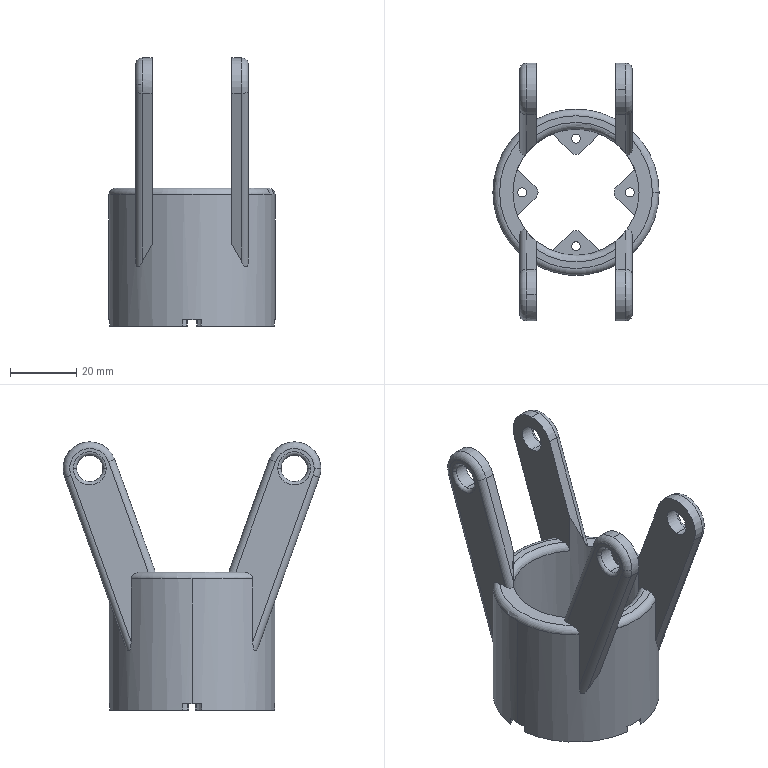Part | SolidWorks | features ICE 7, Fillet 2, CirPattern 1, Extrusion 1, HoleWzd 1 | 1 solid | 130 faces | box 50 x 77.6 x 80.781 mm | volume 47492 mm3 | cylinder 57 | plane 44 | torus 21 | cone 8 | commonest cylinder face diameters 4 x13 7.541 x10 2.7 x8 3.912 x8 8 x8 16 x6